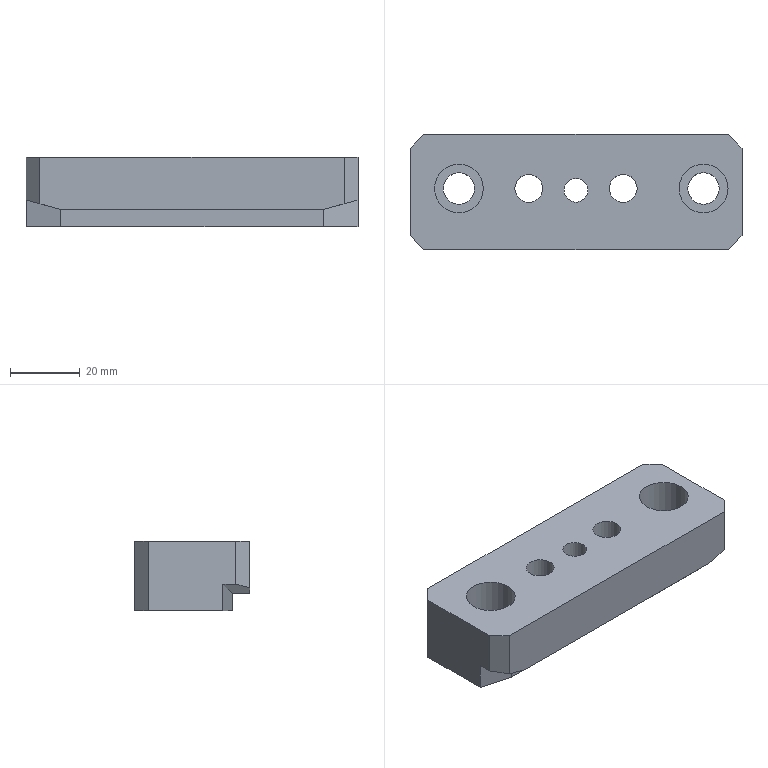Part | NX | features 20 2 | 1 solid | 25 faces | box 95 x 33 x 20 mm | volume 52398 mm3 | plane 18 | cylinder 7 | commonest cylinder face diameters 8.001 x2 9 x2 14 x2 6.8 x1
STEP:
#1=CARTESIAN_POINT('',(3245.002,435.,-3.5));
#2=VERTEX_POINT('',#1);
#3=CARTESIAN_POINT('',(3240.502,435.,-3.5));
#4=DIRECTION('',(0.,0.,-1.));
#5=DIRECTION('',(1.,0.,0.));
#6=AXIS2_PLACEMENT_3D('',#3,#4,#5);
#7=CIRCLE('',#6,4.5);
#8=EDGE_CURVE('',#2,#2,#7,.T.);
#9=ORIENTED_EDGE('',*,*,#8,.F.);
#10=EDGE_LOOP('',(#9));
#11=FACE_BOUND('',#10,.T.);
#12=CARTESIAN_POINT('',(3207.402,434.5,-3.5));
#13=VERTEX_POINT('',#12);
#14=CARTESIAN_POINT('',(3204.002,434.5,-3.5));
#15=DIRECTION('',(0.,0.,-1.));
#16=DIRECTION('',(1.,0.,0.));
#17=AXIS2_PLACEMENT_3D('',#14,#15,#16);
#18=CIRCLE('',#17,3.4);
#19=EDGE_CURVE('',#13,#13,#18,.T.);
#20=ORIENTED_EDGE('',*,*,#19,.F.);
#21=EDGE_LOOP('',(#20));
#22=FACE_BOUND('',#21,.T.);
#23=CARTESIAN_POINT('',(3175.002,435.,-3.5));
#24=VERTEX_POINT('',#23);
#25=CARTESIAN_POINT('',(3170.502,435.,-3.5));
#26=DIRECTION('',(0.,0.,1.));
#27=DIRECTION('',(1.,0.,0.));
#28=AXIS2_PLACEMENT_3D('',#25,#26,#27);
#29=CIRCLE('',#28,4.5);
#30=EDGE_CURVE('',#24,#24,#29,.T.);
#31=ORIENTED_EDGE('',*,*,#30,.T.);
#32=EDGE_LOOP('',(#31));
#33=FACE_BOUND('',#32,.T.);
#34=CARTESIAN_POINT('',(3241.501,422.5,-3.5));
#35=VERTEX_POINT('',#34);
#36=CARTESIAN_POINT('',(3166.501,422.5,-3.5));
#37=VERTEX_POINT('',#36);
#38=CARTESIAN_POINT('',(3222.501,422.5,-3.5));
#39=DIRECTION('',(-1.,0.,0.));
#40=VECTOR('',#39,1000.);
#41=LINE('',#38,#40);
#42=EDGE_CURVE('',#35,#37,#41,.T.);
#43=ORIENTED_EDGE('',*,*,#42,.T.);
#44=CARTESIAN_POINT('',(3156.502,425.179,-3.5));
#45=VERTEX_POINT('',#44);
#46=CARTESIAN_POINT('',(3166.501,422.5,-3.5));
#47=DIRECTION('',(-0.9659,0.2588,0.));
#48=VECTOR('',#47,1000.);
#49=LINE('',#46,#48);
#50=EDGE_CURVE('',#37,#45,#49,.T.);
#51=ORIENTED_EDGE('',*,*,#50,.T.);
#52=CARTESIAN_POINT('',(3156.502,446.5,-3.5));
#53=VERTEX_POINT('',#52);
#54=CARTESIAN_POINT('',(3156.502,417.5,-3.5));
#55=DIRECTION('',(0.,1.,0.));
#56=VECTOR('',#55,1000.);
#57=LINE('',#54,#56);
#58=EDGE_CURVE('',#45,#53,#57,.T.);
#59=ORIENTED_EDGE('',*,*,#58,.T.);
#60=CARTESIAN_POINT('',(3160.502,450.5,-3.5));
#61=VERTEX_POINT('',#60);
#62=CARTESIAN_POINT('',(3160.502,450.5,-3.5));
#63=DIRECTION('',(-0.7071,-0.7071,0.));
#64=VECTOR('',#63,1000.);
#65=LINE('',#62,#64);
#66=EDGE_CURVE('',#61,#53,#65,.T.);
#67=ORIENTED_EDGE('',*,*,#66,.F.);
#68=CARTESIAN_POINT('',(3247.502,450.5,-3.5));
#69=VERTEX_POINT('',#68);
#70=CARTESIAN_POINT('',(3244.502,450.5,-3.5));
#71=DIRECTION('',(1.,0.,0.));
#72=VECTOR('',#71,1000.);
#73=LINE('',#70,#72);
#74=EDGE_CURVE('',#61,#69,#73,.T.);
#75=ORIENTED_EDGE('',*,*,#74,.T.);
#76=CARTESIAN_POINT('',(3251.502,446.5,-3.5));
#77=VERTEX_POINT('',#76);
#78=CARTESIAN_POINT('',(3251.502,446.5,-3.5));
#79=DIRECTION('',(-0.7071,0.7071,0.));
#80=VECTOR('',#79,1000.);
#81=LINE('',#78,#80);
#82=EDGE_CURVE('',#77,#69,#81,.T.);
#83=ORIENTED_EDGE('',*,*,#82,.F.);
#84=CARTESIAN_POINT('',(3251.502,425.18,-3.5));
#85=VERTEX_POINT('',#84);
#86=CARTESIAN_POINT('',(3251.502,450.5,-3.5));
#87=DIRECTION('',(0.,-1.,0.));
#88=VECTOR('',#87,1000.);
#89=LINE('',#86,#88);
#90=EDGE_CURVE('',#77,#85,#89,.T.);
#91=ORIENTED_EDGE('',*,*,#90,.T.);
#92=CARTESIAN_POINT('',(3251.502,425.18,-3.5));
#93=DIRECTION('',(-0.9659,-0.2588,0.));
#94=VECTOR('',#93,1000.);
#95=LINE('',#92,#94);
#96=EDGE_CURVE('',#85,#35,#95,.T.);
#97=ORIENTED_EDGE('',*,*,#96,.T.);
#98=EDGE_LOOP('',(#43,#51,#59,#67,#75,#83,#91,#97));
#99=FACE_BOUND('',#98,.T.);
#100=CARTESIAN_POINT('',(3194.503,435.,-3.5));
#101=VERTEX_POINT('',#100);
#102=CARTESIAN_POINT('',(3190.502,435.,-3.5));
#103=DIRECTION('',(0.,0.,1.));
#104=DIRECTION('',(1.,0.,0.));
#105=AXIS2_PLACEMENT_3D('',#102,#103,#104);
#106=CIRCLE('',#105,4.);
#107=EDGE_CURVE('',#101,#101,#106,.T.);
#108=ORIENTED_EDGE('',*,*,#107,.T.);
#109=EDGE_LOOP('',(#108));
#110=FACE_BOUND('',#109,.T.);
#111=CARTESIAN_POINT('',(3221.503,435.,-3.5));
#112=VERTEX_POINT('',#111);
#113=CARTESIAN_POINT('',(3217.502,435.,-3.5));
#114=DIRECTION('',(0.,0.,-1.));
#115=DIRECTION('',(1.,0.,0.));
#116=AXIS2_PLACEMENT_3D('',#113,#114,#115);
#117=CIRCLE('',#116,4.);
#118=EDGE_CURVE('',#112,#112,#117,.T.);
#119=ORIENTED_EDGE('',*,*,#118,.F.);
#120=EDGE_LOOP('',(#119));
#121=FACE_BOUND('',#120,.T.);
#122=CARTESIAN_POINT('',(3314.502,450.5,-3.5));
#123=DIRECTION('',(0.,0.,1.));
#124=DIRECTION('',(-1.,0.,0.));
#125=AXIS2_PLACEMENT_3D('',#122,#123,#124);
#126=PLANE('',#125);
#127=ADVANCED_FACE('',(#11,#22,#33,#99,#110,#121),#126,.F.);
#128=CARTESIAN_POINT('',(3166.502,417.5,1.5));
#129=VERTEX_POINT('',#128);
#130=CARTESIAN_POINT('',(3241.502,417.5,1.5));
#131=VERTEX_POINT('',#130);
#132=CARTESIAN_POINT('',(3262.502,417.5,1.5));
#133=DIRECTION('',(1.,0.,0.));
#134=VECTOR('',#133,1000.);
#135=LINE('',#132,#134);
#136=EDGE_CURVE('',#129,#131,#135,.T.);
#137=ORIENTED_EDGE('',*,*,#136,.T.);
#138=CARTESIAN_POINT('',(3247.502,417.5,3.108));
#139=VERTEX_POINT('',#138);
#140=CARTESIAN_POINT('',(3241.502,417.5,1.5));
#141=DIRECTION('',(-0.9659,0.,-0.2588));
#142=VECTOR('',#141,1000.);
#143=LINE('',#140,#142);
#144=EDGE_CURVE('',#139,#131,#143,.T.);
#145=ORIENTED_EDGE('',*,*,#144,.F.);
#146=CARTESIAN_POINT('',(3247.502,417.5,16.5));
#147=VERTEX_POINT('',#146);
#148=CARTESIAN_POINT('',(3247.502,417.5,11.5));
#149=DIRECTION('',(0.,0.,-1.));
#150=VECTOR('',#149,1000.);
#151=LINE('',#148,#150);
#152=EDGE_CURVE('',#147,#139,#151,.T.);
#153=ORIENTED_EDGE('',*,*,#152,.F.);
#154=CARTESIAN_POINT('',(3160.502,417.5,16.5));
#155=VERTEX_POINT('',#154);
#156=CARTESIAN_POINT('',(3284.502,417.5,16.5));
#157=DIRECTION('',(-1.,0.,0.));
#158=VECTOR('',#157,1000.);
#159=LINE('',#156,#158);
#160=EDGE_CURVE('',#147,#155,#159,.T.);
#161=ORIENTED_EDGE('',*,*,#160,.T.);
#162=CARTESIAN_POINT('',(3160.502,417.5,3.108));
#163=VERTEX_POINT('',#162);
#164=CARTESIAN_POINT('',(3160.502,417.5,11.5));
#165=DIRECTION('',(0.,0.,1.));
#166=VECTOR('',#165,1000.);
#167=LINE('',#164,#166);
#168=EDGE_CURVE('',#163,#155,#167,.T.);
#169=ORIENTED_EDGE('',*,*,#168,.F.);
#170=CARTESIAN_POINT('',(3166.502,417.5,1.5));
#171=DIRECTION('',(-0.9659,0.,0.2588));
#172=VECTOR('',#171,1000.);
#173=LINE('',#170,#172);
#174=EDGE_CURVE('',#129,#163,#173,.T.);
#175=ORIENTED_EDGE('',*,*,#174,.F.);
#176=EDGE_LOOP('',(#137,#145,#153,#161,#169,#175));
#177=FACE_BOUND('',#176,.T.);
#178=CARTESIAN_POINT('',(3284.502,417.5,11.5));
#179=DIRECTION('',(0.,1.,0.));
#180=DIRECTION('',(0.,0.,1.));
#181=AXIS2_PLACEMENT_3D('',#178,#179,#180);
#182=PLANE('',#181);
#183=ADVANCED_FACE('',(#177),#182,.F.);
#184=CARTESIAN_POINT('',(3221.503,435.,16.5));
#185=VERTEX_POINT('',#184);
#186=CARTESIAN_POINT('',(3217.502,435.,16.5));
#187=DIRECTION('',(0.,0.,1.));
#188=DIRECTION('',(1.,0.,0.));
#189=AXIS2_PLACEMENT_3D('',#186,#187,#188);
#190=CIRCLE('',#189,4.);
#191=EDGE_CURVE('',#185,#185,#190,.T.);
#192=ORIENTED_EDGE('',*,*,#191,.F.);
#193=EDGE_LOOP('',(#192));
#194=FACE_BOUND('',#193,.T.);
#195=CARTESIAN_POINT('',(3194.503,435.,16.5));
#196=VERTEX_POINT('',#195);
#197=CARTESIAN_POINT('',(3190.502,435.,16.5));
#198=DIRECTION('',(0.,0.,1.));
#199=DIRECTION('',(1.,0.,0.));
#200=AXIS2_PLACEMENT_3D('',#197,#198,#199);
#201=CIRCLE('',#200,4.);
#202=EDGE_CURVE('',#196,#196,#201,.T.);
#203=ORIENTED_EDGE('',*,*,#202,.F.);
#204=EDGE_LOOP('',(#203));
#205=FACE_BOUND('',#204,.T.);
#206=CARTESIAN_POINT('',(3247.502,435.,16.5));
#207=VERTEX_POINT('',#206);
#208=CARTESIAN_POINT('',(3240.502,435.,16.5));
#209=DIRECTION('',(0.,0.,-1.));
#210=DIRECTION('',(1.,0.,0.));
#211=AXIS2_PLACEMENT_3D('',#208,#209,#210);
#212=CIRCLE('',#211,7.);
#213=EDGE_CURVE('',#207,#207,#212,.T.);
#214=ORIENTED_EDGE('',*,*,#213,.T.);
#215=EDGE_LOOP('',(#214));
#216=FACE_BOUND('',#215,.T.);
#217=CARTESIAN_POINT('',(3177.502,435.,16.5));
#218=VERTEX_POINT('',#217);
#219=CARTESIAN_POINT('',(3170.502,435.,16.5));
#220=DIRECTION('',(0.,0.,-1.));
#221=DIRECTION('',(1.,0.,0.));
#222=AXIS2_PLACEMENT_3D('',#219,#220,#221);
#223=CIRCLE('',#222,7.);
#224=EDGE_CURVE('',#218,#218,#223,.T.);
#225=ORIENTED_EDGE('',*,*,#224,.T.);
#226=EDGE_LOOP('',(#225));
#227=FACE_BOUND('',#226,.T.);
#228=ORIENTED_EDGE('',*,*,#160,.F.);
#229=CARTESIAN_POINT('',(3251.502,421.5,16.5));
#230=VERTEX_POINT('',#229);
#231=CARTESIAN_POINT('',(3247.502,417.5,16.5));
#232=DIRECTION('',(-0.7071,-0.7071,0.));
#233=VECTOR('',#232,1000.);
#234=LINE('',#231,#233);
#235=EDGE_CURVE('',#230,#147,#234,.T.);
#236=ORIENTED_EDGE('',*,*,#235,.F.);
#237=CARTESIAN_POINT('',(3251.502,446.5,16.5));
#238=VERTEX_POINT('',#237);
#239=CARTESIAN_POINT('',(3251.502,450.5,16.5));
#240=DIRECTION('',(0.,-1.,0.));
#241=VECTOR('',#240,1000.);
#242=LINE('',#239,#241);
#243=EDGE_CURVE('',#238,#230,#242,.T.);
#244=ORIENTED_EDGE('',*,*,#243,.F.);
#245=CARTESIAN_POINT('',(3247.502,450.5,16.5));
#246=VERTEX_POINT('',#245);
#247=CARTESIAN_POINT('',(3251.502,446.5,16.5));
#248=DIRECTION('',(0.7071,-0.7071,0.));
#249=VECTOR('',#248,1000.);
#250=LINE('',#247,#249);
#251=EDGE_CURVE('',#246,#238,#250,.T.);
#252=ORIENTED_EDGE('',*,*,#251,.F.);
#253=CARTESIAN_POINT('',(3160.502,450.5,16.5));
#254=VERTEX_POINT('',#253);
#255=CARTESIAN_POINT('',(3204.502,450.5,16.5));
#256=DIRECTION('',(1.,0.,0.));
#257=VECTOR('',#256,1000.);
#258=LINE('',#255,#257);
#259=EDGE_CURVE('',#254,#246,#258,.T.);
#260=ORIENTED_EDGE('',*,*,#259,.F.);
#261=CARTESIAN_POINT('',(3156.502,446.5,16.5));
#262=VERTEX_POINT('',#261);
#263=CARTESIAN_POINT('',(3160.502,450.5,16.5));
#264=DIRECTION('',(0.7071,0.7071,0.));
#265=VECTOR('',#264,1000.);
#266=LINE('',#263,#265);
#267=EDGE_CURVE('',#262,#254,#266,.T.);
#268=ORIENTED_EDGE('',*,*,#267,.F.);
#269=CARTESIAN_POINT('',(3156.502,421.5,16.5));
#270=VERTEX_POINT('',#269);
#271=CARTESIAN_POINT('',(3156.502,417.5,16.5));
#272=DIRECTION('',(0.,1.,0.));
#273=VECTOR('',#272,1000.);
#274=LINE('',#271,#273);
#275=EDGE_CURVE('',#270,#262,#274,.T.);
#276=ORIENTED_EDGE('',*,*,#275,.F.);
#277=CARTESIAN_POINT('',(3156.502,421.5,16.5));
#278=DIRECTION('',(-0.7071,0.7071,0.));
#279=VECTOR('',#278,1000.);
#280=LINE('',#277,#279);
#281=EDGE_CURVE('',#155,#270,#280,.T.);
#282=ORIENTED_EDGE('',*,*,#281,.F.);
#283=EDGE_LOOP('',(#228,#236,#244,#252,#260,#268,#276,#282));
#284=FACE_BOUND('',#283,.T.);
#285=CARTESIAN_POINT('',(3207.402,434.5,16.5));
#286=VERTEX_POINT('',#285);
#287=CARTESIAN_POINT('',(3204.002,434.5,16.5));
#288=DIRECTION('',(0.,0.,1.));
#289=DIRECTION('',(1.,0.,0.));
#290=AXIS2_PLACEMENT_3D('',#287,#288,#289);
#291=CIRCLE('',#290,3.4);
#292=EDGE_CURVE('',#286,#286,#291,.T.);
#293=ORIENTED_EDGE('',*,*,#292,.F.);
#294=EDGE_LOOP('',(#293));
#295=FACE_BOUND('',#294,.T.);
#296=CARTESIAN_POINT('',(3284.502,450.5,16.5));
#297=DIRECTION('',(0.,0.,1.));
#298=DIRECTION('',(-1.,0.,0.));
#299=AXIS2_PLACEMENT_3D('',#296,#297,#298);
#300=PLANE('',#299);
#301=ADVANCED_FACE('',(#194,#205,#216,#227,#284,#295),#300,.T.);
#302=CARTESIAN_POINT('',(3236.002,435.,6.5));
#303=VERTEX_POINT('',#302);
#304=CARTESIAN_POINT('',(3240.502,435.,6.5));
#305=DIRECTION('',(0.,0.,1.));
#306=DIRECTION('',(-1.,0.,0.));
#307=AXIS2_PLACEMENT_3D('',#304,#305,#306);
#308=CIRCLE('',#307,4.5);
#309=EDGE_CURVE('',#303,#303,#308,.T.);
#310=ORIENTED_EDGE('',*,*,#309,.F.);
#311=EDGE_LOOP('',(#310));
#312=FACE_BOUND('',#311,.T.);
#313=CARTESIAN_POINT('',(3233.502,435.,6.5));
#314=VERTEX_POINT('',#313);
#315=CARTESIAN_POINT('',(3240.502,435.,6.5));
#316=DIRECTION('',(0.,0.,-1.));
#317=DIRECTION('',(-1.,0.,0.));
#318=AXIS2_PLACEMENT_3D('',#315,#316,#317);
#319=CIRCLE('',#318,7.);
#320=EDGE_CURVE('',#314,#314,#319,.T.);
#321=ORIENTED_EDGE('',*,*,#320,.F.);
#322=EDGE_LOOP('',(#321));
#323=FACE_BOUND('',#322,.T.);
#324=CARTESIAN_POINT('',(3240.502,432.5,6.5));
#325=DIRECTION('',(0.,0.,-1.));
#326=DIRECTION('',(1.,0.,0.));
#327=AXIS2_PLACEMENT_3D('',#324,#325,#326);
#328=PLANE('',#327);
#329=ADVANCED_FACE('',(#312,#323),#328,.F.);
#330=CARTESIAN_POINT('',(3241.502,422.5,1.5));
#331=VERTEX_POINT('',#330);
#332=CARTESIAN_POINT('',(3241.502,425.18,1.5));
#333=DIRECTION('',(0.,1.,0.));
#334=VECTOR('',#333,1000.);
#335=LINE('',#332,#334);
#336=EDGE_CURVE('',#131,#331,#335,.T.);
#337=ORIENTED_EDGE('',*,*,#336,.T.);
#338=CARTESIAN_POINT('',(3251.502,425.18,4.179));
#339=VERTEX_POINT('',#338);
#340=CARTESIAN_POINT('',(3250.875,425.012,4.011));
#341=DIRECTION('',(0.9351,0.2506,0.2506));
#342=VECTOR('',#341,1000.);
#343=LINE('',#340,#342);
#344=EDGE_CURVE('',#331,#339,#343,.T.);
#345=ORIENTED_EDGE('',*,*,#344,.T.);
#346=CARTESIAN_POINT('',(3251.502,421.5,4.179));
#347=VERTEX_POINT('',#346);
#348=CARTESIAN_POINT('',(3251.502,417.5,4.179));
#349=DIRECTION('',(0.,-1.,0.));
#350=VECTOR('',#349,1000.);
#351=LINE('',#348,#350);
#352=EDGE_CURVE('',#339,#347,#351,.T.);
#353=ORIENTED_EDGE('',*,*,#352,.T.);
#354=CARTESIAN_POINT('',(3234.451,404.449,-0.3894));
#355=DIRECTION('',(0.6947,0.6947,0.1862));
#356=VECTOR('',#355,1000.);
#357=LINE('',#354,#356);
#358=EDGE_CURVE('',#139,#347,#357,.T.);
#359=ORIENTED_EDGE('',*,*,#358,.F.);
#360=ORIENTED_EDGE('',*,*,#144,.T.);
#361=EDGE_LOOP('',(#337,#345,#353,#359,#360));
#362=FACE_BOUND('',#361,.T.);
#363=CARTESIAN_POINT('',(3241.502,396.891,1.5));
#364=DIRECTION('',(0.2588,0.,-0.9659));
#365=DIRECTION('',(0.9659,0.,0.2588));
#366=AXIS2_PLACEMENT_3D('',#363,#364,#365);
#367=PLANE('',#366);
#368=ADVANCED_FACE('',(#362),#367,.T.);
#369=CARTESIAN_POINT('',(3166.002,435.,6.5));
#370=VERTEX_POINT('',#369);
#371=CARTESIAN_POINT('',(3170.502,435.,6.5));
#372=DIRECTION('',(0.,0.,1.));
#373=DIRECTION('',(-1.,0.,0.));
#374=AXIS2_PLACEMENT_3D('',#371,#372,#373);
#375=CIRCLE('',#374,4.5);
#376=EDGE_CURVE('',#370,#370,#375,.T.);
#377=ORIENTED_EDGE('',*,*,#376,.F.);
#378=EDGE_LOOP('',(#377));
#379=FACE_BOUND('',#378,.T.);
#380=CARTESIAN_POINT('',(3163.502,435.,6.5));
#381=VERTEX_POINT('',#380);
#382=CARTESIAN_POINT('',(3170.502,435.,6.5));
#383=DIRECTION('',(0.,0.,-1.));
#384=DIRECTION('',(-1.,0.,0.));
#385=AXIS2_PLACEMENT_3D('',#382,#383,#384);
#386=CIRCLE('',#385,7.);
#387=EDGE_CURVE('',#381,#381,#386,.T.);
#388=ORIENTED_EDGE('',*,*,#387,.F.);
#389=EDGE_LOOP('',(#388));
#390=FACE_BOUND('',#389,.T.);
#391=CARTESIAN_POINT('',(3170.502,432.5,6.5));
#392=DIRECTION('',(0.,0.,-1.));
#393=DIRECTION('',(-1.,0.,0.));
#394=AXIS2_PLACEMENT_3D('',#391,#392,#393);
#395=PLANE('',#394);
#396=ADVANCED_FACE('',(#379,#390),#395,.F.);
#397=ORIENTED_EDGE('',*,*,#213,.F.);
#398=EDGE_LOOP('',(#397));
#399=FACE_BOUND('',#398,.T.);
#400=ORIENTED_EDGE('',*,*,#320,.T.);
#401=EDGE_LOOP('',(#400));
#402=FACE_BOUND('',#401,.T.);
#403=CARTESIAN_POINT('',(3240.502,435.,42.5));
#404=DIRECTION('',(0.,0.,-1.));
#405=DIRECTION('',(1.,0.,0.));
#406=AXIS2_PLACEMENT_3D('',#403,#404,#405);
#407=CYLINDRICAL_SURFACE('',#406,7.);
#408=ADVANCED_FACE('',(#399,#402),#407,.F.);
#409=ORIENTED_EDGE('',*,*,#235,.T.);
#410=ORIENTED_EDGE('',*,*,#152,.T.);
#411=ORIENTED_EDGE('',*,*,#358,.T.);
#412=CARTESIAN_POINT('',(3251.502,421.5,11.5));
#413=DIRECTION('',(0.,0.,1.));
#414=VECTOR('',#413,1000.);
#415=LINE('',#412,#414);
#416=EDGE_CURVE('',#347,#230,#415,.T.);
#417=ORIENTED_EDGE('',*,*,#416,.T.);
#418=EDGE_LOOP('',(#409,#410,#411,#417));
#419=FACE_BOUND('',#418,.T.);
#420=CARTESIAN_POINT('',(3247.502,417.5,11.5));
#421=DIRECTION('',(-0.7071,0.7071,0.));
#422=DIRECTION('',(0.,0.,-1.));
#423=AXIS2_PLACEMENT_3D('',#420,#421,#422);
#424=PLANE('',#423);
#425=ADVANCED_FACE('',(#419),#424,.F.);
#426=ORIENTED_EDGE('',*,*,#387,.T.);
#427=EDGE_LOOP('',(#426));
#428=FACE_BOUND('',#427,.T.);
#429=ORIENTED_EDGE('',*,*,#224,.F.);
#430=EDGE_LOOP('',(#429));
#431=FACE_BOUND('',#430,.T.);
#432=CARTESIAN_POINT('',(3170.502,435.,42.5));
#433=DIRECTION('',(0.,0.,-1.));
#434=DIRECTION('',(-1.,0.,0.));
#435=AXIS2_PLACEMENT_3D('',#432,#433,#434);
#436=CYLINDRICAL_SURFACE('',#435,7.);
#437=ADVANCED_FACE('',(#428,#431),#436,.F.);
#438=ORIENTED_EDGE('',*,*,#352,.F.);
#439=CARTESIAN_POINT('',(3251.502,425.18,3.5));
#440=DIRECTION('',(0.,0.,-1.));
#441=VECTOR('',#440,1000.);
#442=LINE('',#439,#441);
#443=EDGE_CURVE('',#339,#85,#442,.T.);
#444=ORIENTED_EDGE('',*,*,#443,.T.);
#445=ORIENTED_EDGE('',*,*,#90,.F.);
#446=CARTESIAN_POINT('',(3251.502,446.5,11.5));
#447=DIRECTION('',(0.,0.,-1.));
#448=VECTOR('',#447,1000.);
#449=LINE('',#446,#448);
#450=EDGE_CURVE('',#238,#77,#449,.T.);
#451=ORIENTED_EDGE('',*,*,#450,.F.);
#452=ORIENTED_EDGE('',*,*,#243,.T.);
#453=ORIENTED_EDGE('',*,*,#416,.F.);
#454=EDGE_LOOP('',(#438,#444,#445,#451,#452,#453));
#455=FACE_BOUND('',#454,.T.);
#456=CARTESIAN_POINT('',(3251.502,450.5,11.5));
#457=DIRECTION('',(-1.,0.,0.));
#458=DIRECTION('',(0.,0.,-1.));
#459=AXIS2_PLACEMENT_3D('',#456,#457,#458);
#460=PLANE('',#459);
#461=ADVANCED_FACE('',(#455),#460,.F.);
#462=CARTESIAN_POINT('',(3241.501,422.5,1.5));
#463=VERTEX_POINT('',#462);
#464=CARTESIAN_POINT('',(3251.502,425.18,1.5));
#465=DIRECTION('',(0.9659,0.2588,0.));
#466=VECTOR('',#465,1000.);
#467=LINE('',#464,#466);
#468=EDGE_CURVE('',#463,#331,#467,.T.);
#469=ORIENTED_EDGE('',*,*,#468,.F.);
#470=CARTESIAN_POINT('',(3241.501,422.5,3.5));
#471=DIRECTION('',(0.,0.,1.));
#472=VECTOR('',#471,1000.);
#473=LINE('',#470,#472);
#474=EDGE_CURVE('',#35,#463,#473,.T.);
#475=ORIENTED_EDGE('',*,*,#474,.F.);
#476=ORIENTED_EDGE('',*,*,#96,.F.);
#477=ORIENTED_EDGE('',*,*,#443,.F.);
#478=ORIENTED_EDGE('',*,*,#344,.F.);
#479=EDGE_LOOP('',(#469,#475,#476,#477,#478));
#480=FACE_BOUND('',#479,.T.);
#481=CARTESIAN_POINT('',(3251.502,425.18,3.5));
#482=DIRECTION('',(-0.2588,0.9659,0.));
#483=DIRECTION('',(0.9659,0.2588,0.));
#484=AXIS2_PLACEMENT_3D('',#481,#482,#483);
#485=PLANE('',#484);
#486=ADVANCED_FACE('',(#480),#485,.F.);
#487=ORIENTED_EDGE('',*,*,#309,.T.);
#488=EDGE_LOOP('',(#487));
#489=FACE_BOUND('',#488,.T.);
#490=ORIENTED_EDGE('',*,*,#8,.T.);
#491=EDGE_LOOP('',(#490));
#492=FACE_BOUND('',#491,.T.);
#493=CARTESIAN_POINT('',(3240.502,435.,42.5));
#494=DIRECTION('',(0.,0.,-1.));
#495=DIRECTION('',(1.,0.,0.));
#496=AXIS2_PLACEMENT_3D('',#493,#494,#495);
#497=CYLINDRICAL_SURFACE('',#496,4.5);
#498=ADVANCED_FACE('',(#489,#492),#497,.F.);
#499=ORIENTED_EDGE('',*,*,#474,.T.);
#500=CARTESIAN_POINT('',(3166.502,422.5,1.5));
#501=VERTEX_POINT('',#500);
#502=CARTESIAN_POINT('',(3252.501,422.5,1.5));
#503=DIRECTION('',(1.,0.,0.));
#504=VECTOR('',#503,1000.);
#505=LINE('',#502,#504);
#506=EDGE_CURVE('',#501,#463,#505,.T.);
#507=ORIENTED_EDGE('',*,*,#506,.F.);
#508=CARTESIAN_POINT('',(3166.501,422.5,1.5));
#509=VERTEX_POINT('',#508);
#510=CARTESIAN_POINT('',(3166.502,422.5,1.5));
#511=DIRECTION('',(0.9659,0.,-0.2588));
#512=VECTOR('',#511,1000.);
#513=LINE('',#510,#512);
#514=EDGE_CURVE('',#509,#501,#513,.T.);
#515=ORIENTED_EDGE('',*,*,#514,.F.);
#516=CARTESIAN_POINT('',(3166.501,422.5,3.5));
#517=DIRECTION('',(0.,0.,1.));
#518=VECTOR('',#517,1000.);
#519=LINE('',#516,#518);
#520=EDGE_CURVE('',#37,#509,#519,.T.);
#521=ORIENTED_EDGE('',*,*,#520,.F.);
#522=ORIENTED_EDGE('',*,*,#42,.F.);
#523=EDGE_LOOP('',(#499,#507,#515,#521,#522));
#524=FACE_BOUND('',#523,.T.);
#525=CARTESIAN_POINT('',(3184.501,422.5,3.5));
#526=DIRECTION('',(0.,1.,0.));
#527=DIRECTION('',(0.,0.,1.));
#528=AXIS2_PLACEMENT_3D('',#525,#526,#527);
#529=PLANE('',#528);
#530=ADVANCED_FACE('',(#524),#529,.F.);
#531=CARTESIAN_POINT('',(3156.502,421.5,4.179));
#532=VERTEX_POINT('',#531);
#533=CARTESIAN_POINT('',(3156.502,421.5,11.5));
#534=DIRECTION('',(0.,0.,-1.));
#535=VECTOR('',#534,1000.);
#536=LINE('',#533,#535);
#537=EDGE_CURVE('',#270,#532,#536,.T.);
#538=ORIENTED_EDGE('',*,*,#537,.T.);
#539=CARTESIAN_POINT('',(3173.554,404.449,-0.3894));
#540=DIRECTION('',(0.6947,-0.6947,-0.1862));
#541=VECTOR('',#540,1000.);
#542=LINE('',#539,#541);
#543=EDGE_CURVE('',#532,#163,#542,.T.);
#544=ORIENTED_EDGE('',*,*,#543,.T.);
#545=ORIENTED_EDGE('',*,*,#168,.T.);
#546=ORIENTED_EDGE('',*,*,#281,.T.);
#547=EDGE_LOOP('',(#538,#544,#545,#546));
#548=FACE_BOUND('',#547,.T.);
#549=CARTESIAN_POINT('',(3156.502,421.5,11.5));
#550=DIRECTION('',(0.7071,0.7071,0.));
#551=DIRECTION('',(0.,0.,-1.));
#552=AXIS2_PLACEMENT_3D('',#549,#550,#551);
#553=PLANE('',#552);
#554=ADVANCED_FACE('',(#548),#553,.F.);
#555=ORIENTED_EDGE('',*,*,#30,.F.);
#556=EDGE_LOOP('',(#555));
#557=FACE_BOUND('',#556,.T.);
#558=ORIENTED_EDGE('',*,*,#376,.T.);
#559=EDGE_LOOP('',(#558));
#560=FACE_BOUND('',#559,.T.);
#561=CARTESIAN_POINT('',(3170.502,435.,42.5));
#562=DIRECTION('',(0.,0.,-1.));
#563=DIRECTION('',(-1.,0.,0.));
#564=AXIS2_PLACEMENT_3D('',#561,#562,#563);
#565=CYLINDRICAL_SURFACE('',#564,4.5);
#566=ADVANCED_FACE('',(#557,#560),#565,.F.);
#567=ORIENTED_EDGE('',*,*,#58,.F.);
#568=CARTESIAN_POINT('',(3156.502,425.179,4.179));
#569=VERTEX_POINT('',#568);
#570=CARTESIAN_POINT('',(3156.502,425.179,3.5));
#571=DIRECTION('',(0.,0.,-1.));
#572=VECTOR('',#571,1000.);
#573=LINE('',#570,#572);
#574=EDGE_CURVE('',#569,#45,#573,.T.);
#575=ORIENTED_EDGE('',*,*,#574,.F.);
#576=CARTESIAN_POINT('',(3156.502,425.179,4.179));
#577=DIRECTION('',(0.,1.,0.));
#578=VECTOR('',#577,1000.);
#579=LINE('',#576,#578);
#580=EDGE_CURVE('',#532,#569,#579,.T.);
#581=ORIENTED_EDGE('',*,*,#580,.F.);
#582=ORIENTED_EDGE('',*,*,#537,.F.);
#583=ORIENTED_EDGE('',*,*,#275,.T.);
#584=CARTESIAN_POINT('',(3156.502,446.5,11.5));
#585=DIRECTION('',(0.,0.,1.));
#586=VECTOR('',#585,1000.);
#587=LINE('',#584,#586);
#588=EDGE_CURVE('',#53,#262,#587,.T.);
#589=ORIENTED_EDGE('',*,*,#588,.F.);
#590=EDGE_LOOP('',(#567,#575,#581,#582,#583,#589));
#591=FACE_BOUND('',#590,.T.);
#592=CARTESIAN_POINT('',(3156.502,417.5,11.5));
#593=DIRECTION('',(1.,0.,0.));
#594=DIRECTION('',(0.,0.,1.));
#595=AXIS2_PLACEMENT_3D('',#592,#593,#594);
#596=PLANE('',#595);
#597=ADVANCED_FACE('',(#591),#596,.F.);
#598=ORIENTED_EDGE('',*,*,#580,.T.);
#599=CARTESIAN_POINT('',(3166.501,422.5,1.5));
#600=DIRECTION('',(0.9351,-0.2506,-0.2506));
#601=VECTOR('',#600,1000.);
#602=LINE('',#599,#601);
#603=EDGE_CURVE('',#569,#509,#602,.T.);
#604=ORIENTED_EDGE('',*,*,#603,.T.);
#605=ORIENTED_EDGE('',*,*,#514,.T.);
#606=CARTESIAN_POINT('',(3166.502,417.5,1.5));
#607=DIRECTION('',(0.,-1.,0.));
#608=VECTOR('',#607,1000.);
#609=LINE('',#606,#608);
#610=EDGE_CURVE('',#501,#129,#609,.T.);
#611=ORIENTED_EDGE('',*,*,#610,.T.);
#612=ORIENTED_EDGE('',*,*,#174,.T.);
#613=ORIENTED_EDGE('',*,*,#543,.F.);
#614=EDGE_LOOP('',(#598,#604,#605,#611,#612,#613));
#615=FACE_BOUND('',#614,.T.);
#616=CARTESIAN_POINT('',(3166.502,396.891,1.5));
#617=DIRECTION('',(-0.2588,0.,-0.9659));
#618=DIRECTION('',(0.9659,0.,-0.2588));
#619=AXIS2_PLACEMENT_3D('',#616,#617,#618);
#620=PLANE('',#619);
#621=ADVANCED_FACE('',(#615),#620,.T.);
#622=ORIENTED_EDGE('',*,*,#50,.F.);
#623=ORIENTED_EDGE('',*,*,#520,.T.);
#624=ORIENTED_EDGE('',*,*,#603,.F.);
#625=ORIENTED_EDGE('',*,*,#574,.T.);
#626=EDGE_LOOP('',(#622,#623,#624,#625));
#627=FACE_BOUND('',#626,.T.);
#628=CARTESIAN_POINT('',(3166.501,422.5,3.5));
#629=DIRECTION('',(0.2588,0.9659,0.));
#630=DIRECTION('',(0.9659,-0.2588,0.));
#631=AXIS2_PLACEMENT_3D('',#628,#629,#630);
#632=PLANE('',#631);
#633=ADVANCED_FACE('',(#627),#632,.F.);
#634=ORIENTED_EDGE('',*,*,#66,.T.);
#635=ORIENTED_EDGE('',*,*,#588,.T.);
#636=ORIENTED_EDGE('',*,*,#267,.T.);
#637=CARTESIAN_POINT('',(3160.502,450.5,11.5));
#638=DIRECTION('',(0.,0.,-1.));
#639=VECTOR('',#638,1000.);
#640=LINE('',#637,#639);
#641=EDGE_CURVE('',#254,#61,#640,.T.);
#642=ORIENTED_EDGE('',*,*,#641,.T.);
#643=EDGE_LOOP('',(#634,#635,#636,#642));
#644=FACE_BOUND('',#643,.T.);
#645=CARTESIAN_POINT('',(3160.502,450.5,11.5));
#646=DIRECTION('',(0.7071,-0.7071,0.));
#647=DIRECTION('',(0.,0.,-1.));
#648=AXIS2_PLACEMENT_3D('',#645,#646,#647);
#649=PLANE('',#648);
#650=ADVANCED_FACE('',(#644),#649,.F.);
#651=ORIENTED_EDGE('',*,*,#82,.T.);
#652=CARTESIAN_POINT('',(3247.502,450.5,11.5));
#653=DIRECTION('',(0.,0.,1.));
#654=VECTOR('',#653,1000.);
#655=LINE('',#652,#654);
#656=EDGE_CURVE('',#69,#246,#655,.T.);
#657=ORIENTED_EDGE('',*,*,#656,.T.);
#658=ORIENTED_EDGE('',*,*,#251,.T.);
#659=ORIENTED_EDGE('',*,*,#450,.T.);
#660=EDGE_LOOP('',(#651,#657,#658,#659));
#661=FACE_BOUND('',#660,.T.);
#662=CARTESIAN_POINT('',(3251.502,446.5,11.5));
#663=DIRECTION('',(-0.7071,-0.7071,0.));
#664=DIRECTION('',(0.,0.,-1.));
#665=AXIS2_PLACEMENT_3D('',#662,#663,#664);
#666=PLANE('',#665);
#667=ADVANCED_FACE('',(#661),#666,.F.);
#668=ORIENTED_EDGE('',*,*,#656,.F.);
#669=ORIENTED_EDGE('',*,*,#74,.F.);
#670=ORIENTED_EDGE('',*,*,#641,.F.);
#671=ORIENTED_EDGE('',*,*,#259,.T.);
#672=EDGE_LOOP('',(#668,#669,#670,#671));
#673=FACE_BOUND('',#672,.T.);
#674=CARTESIAN_POINT('',(3204.502,450.5,11.5));
#675=DIRECTION('',(0.,-1.,0.));
#676=DIRECTION('',(0.,0.,-1.));
#677=AXIS2_PLACEMENT_3D('',#674,#675,#676);
#678=PLANE('',#677);
#679=ADVANCED_FACE('',(#673),#678,.F.);
#680=ORIENTED_EDGE('',*,*,#506,.T.);
#681=ORIENTED_EDGE('',*,*,#468,.T.);
#682=ORIENTED_EDGE('',*,*,#336,.F.);
#683=ORIENTED_EDGE('',*,*,#136,.F.);
#684=ORIENTED_EDGE('',*,*,#610,.F.);
#685=EDGE_LOOP('',(#680,#681,#682,#683,#684));
#686=FACE_BOUND('',#685,.T.);
#687=CARTESIAN_POINT('',(3284.773,396.891,1.5));
#688=DIRECTION('',(0.,0.,-1.));
#689=DIRECTION('',(1.,0.,0.));
#690=AXIS2_PLACEMENT_3D('',#687,#688,#689);
#691=PLANE('',#690);
#692=ADVANCED_FACE('',(#686),#691,.T.);
#693=ORIENTED_EDGE('',*,*,#292,.T.);
#694=EDGE_LOOP('',(#693));
#695=FACE_BOUND('',#694,.T.);
#696=ORIENTED_EDGE('',*,*,#19,.T.);
#697=EDGE_LOOP('',(#696));
#698=FACE_BOUND('',#697,.T.);
#699=CARTESIAN_POINT('',(3204.002,434.5,16.5));
#700=DIRECTION('',(0.,0.,-1.));
#701=DIRECTION('',(-1.,0.,0.));
#702=AXIS2_PLACEMENT_3D('',#699,#700,#701);
#703=CYLINDRICAL_SURFACE('',#702,3.4);
#704=ADVANCED_FACE('',(#695,#698),#703,.F.);
#705=ORIENTED_EDGE('',*,*,#202,.T.);
#706=EDGE_LOOP('',(#705));
#707=FACE_BOUND('',#706,.T.);
#708=ORIENTED_EDGE('',*,*,#107,.F.);
#709=EDGE_LOOP('',(#708));
#710=FACE_BOUND('',#709,.T.);
#711=CARTESIAN_POINT('',(3190.502,435.,-3.5));
#712=DIRECTION('',(0.,0.,1.));
#713=DIRECTION('',(-1.,0.,0.));
#714=AXIS2_PLACEMENT_3D('',#711,#712,#713);
#715=CYLINDRICAL_SURFACE('',#714,4.);
#716=ADVANCED_FACE('',(#707,#710),#715,.F.);
#717=ORIENTED_EDGE('',*,*,#191,.T.);
#718=EDGE_LOOP('',(#717));
#719=FACE_BOUND('',#718,.T.);
#720=ORIENTED_EDGE('',*,*,#118,.T.);
#721=EDGE_LOOP('',(#720));
#722=FACE_BOUND('',#721,.T.);
#723=CARTESIAN_POINT('',(3217.502,435.,-3.5));
#724=DIRECTION('',(0.,0.,1.));
#725=DIRECTION('',(1.,0.,0.));
#726=AXIS2_PLACEMENT_3D('',#723,#724,#725);
#727=CYLINDRICAL_SURFACE('',#726,4.);
#728=ADVANCED_FACE('',(#719,#722),#727,.F.);
#729=CLOSED_SHELL('',(#127,#183,#301,#329,#368,#396,#408,#425,#437,#461,#486,#498,#530,#554,#566,#597,#621,#633,#650,#667,#679,#692,#704,#716,#728));
#730=MANIFOLD_SOLID_BREP('',#729);
#731=(LENGTH_UNIT()NAMED_UNIT(*)SI_UNIT(.MILLI.,.METRE.));
#732=UNCERTAINTY_MEASURE_WITH_UNIT(LENGTH_MEASURE(0.00001),#731,'','');
#733=(NAMED_UNIT(*)PLANE_ANGLE_UNIT()SI_UNIT($,.RADIAN.));
#734=(NAMED_UNIT(*)SI_UNIT($,.STERADIAN.)SOLID_ANGLE_UNIT());
#735=(GEOMETRIC_REPRESENTATION_CONTEXT(3)GLOBAL_UNCERTAINTY_ASSIGNED_CONTEXT((#732))GLOBAL_UNIT_ASSIGNED_CONTEXT((#731,#733,#734))REPRESENTATION_CONTEXT('',''));
#736=ADVANCED_BREP_SHAPE_REPRESENTATION('',(#730),#735);